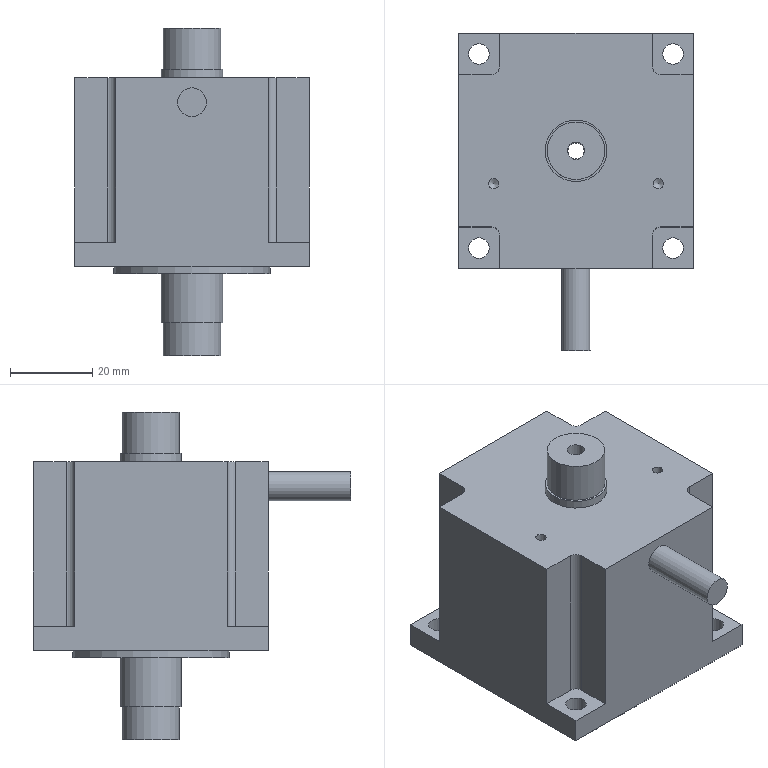Part | NX | 1 solid | 45 faces | box 57 x 77 x 79.6 mm | volume 139845 mm3 | plane 24 | cylinder 18 | cone 3 | commonest cylinder face diameters 4 x5 5 x4 2.5 x2 14 x2 15 x2 4.2 x1
STEP:
#1=CARTESIAN_POINT('',(18.5,-28.5,6.));
#2=VERTEX_POINT('',#1);
#3=CARTESIAN_POINT('',(28.5,-28.5,6.));
#4=VERTEX_POINT('',#3);
#5=CARTESIAN_POINT('',(28.5,-28.5,6.));
#6=DIRECTION('',(1.,0.,0.));
#7=VECTOR('',#6,1000.);
#8=LINE('',#5,#7);
#9=EDGE_CURVE('',#2,#4,#8,.T.);
#10=ORIENTED_EDGE('',*,*,#9,.F.);
#11=CARTESIAN_POINT('',(18.5,-28.5,46.));
#12=VERTEX_POINT('',#11);
#13=CARTESIAN_POINT('',(18.5,-28.5,6.));
#14=DIRECTION('',(0.,0.,1.));
#15=VECTOR('',#14,1000.);
#16=LINE('',#13,#15);
#17=EDGE_CURVE('',#2,#12,#16,.T.);
#18=ORIENTED_EDGE('',*,*,#17,.T.);
#19=CARTESIAN_POINT('',(-18.5,-28.5,46.));
#20=VERTEX_POINT('',#19);
#21=CARTESIAN_POINT('',(-28.5,-28.5,46.));
#22=DIRECTION('',(1.,0.,0.));
#23=VECTOR('',#22,1000.);
#24=LINE('',#21,#23);
#25=EDGE_CURVE('',#20,#12,#24,.T.);
#26=ORIENTED_EDGE('',*,*,#25,.F.);
#27=CARTESIAN_POINT('',(-18.5,-28.5,6.));
#28=VERTEX_POINT('',#27);
#29=CARTESIAN_POINT('',(-18.5,-28.5,6.));
#30=DIRECTION('',(0.,0.,1.));
#31=VECTOR('',#30,1000.);
#32=LINE('',#29,#31);
#33=EDGE_CURVE('',#28,#20,#32,.T.);
#34=ORIENTED_EDGE('',*,*,#33,.F.);
#35=CARTESIAN_POINT('',(-28.5,-28.5,6.));
#36=VERTEX_POINT('',#35);
#37=CARTESIAN_POINT('',(-28.5,-28.5,6.));
#38=DIRECTION('',(1.,0.,0.));
#39=VECTOR('',#38,1000.);
#40=LINE('',#37,#39);
#41=EDGE_CURVE('',#36,#28,#40,.T.);
#42=ORIENTED_EDGE('',*,*,#41,.F.);
#43=CARTESIAN_POINT('',(-28.5,-28.5,0.));
#44=VERTEX_POINT('',#43);
#45=CARTESIAN_POINT('',(-28.5,-28.5,46.));
#46=DIRECTION('',(0.,0.,-1.));
#47=VECTOR('',#46,1000.);
#48=LINE('',#45,#47);
#49=EDGE_CURVE('',#36,#44,#48,.T.);
#50=ORIENTED_EDGE('',*,*,#49,.T.);
#51=CARTESIAN_POINT('',(28.5,-28.5,0.));
#52=VERTEX_POINT('',#51);
#53=CARTESIAN_POINT('',(-28.5,-28.5,0.));
#54=DIRECTION('',(1.,0.,0.));
#55=VECTOR('',#54,1000.);
#56=LINE('',#53,#55);
#57=EDGE_CURVE('',#44,#52,#56,.T.);
#58=ORIENTED_EDGE('',*,*,#57,.T.);
#59=CARTESIAN_POINT('',(28.5,-28.5,46.));
#60=DIRECTION('',(0.,0.,-1.));
#61=VECTOR('',#60,1000.);
#62=LINE('',#59,#61);
#63=EDGE_CURVE('',#4,#52,#62,.T.);
#64=ORIENTED_EDGE('',*,*,#63,.F.);
#65=EDGE_LOOP('',(#10,#18,#26,#34,#42,#50,#58,#64));
#66=FACE_BOUND('',#65,.T.);
#67=CARTESIAN_POINT('',(0.,-28.5,43.5));
#68=VERTEX_POINT('',#67);
#69=CARTESIAN_POINT('',(0.,-28.5,40.));
#70=DIRECTION('',(0.,1.,0.));
#71=DIRECTION('',(0.,0.,1.));
#72=AXIS2_PLACEMENT_3D('',#69,#70,#71);
#73=CIRCLE('',#72,3.5);
#74=EDGE_CURVE('',#68,#68,#73,.F.);
#75=ORIENTED_EDGE('',*,*,#74,.F.);
#76=EDGE_LOOP('',(#75));
#77=FACE_BOUND('',#76,.T.);
#78=CARTESIAN_POINT('',(-28.5,-28.5,46.));
#79=DIRECTION('',(0.,1.,0.));
#80=DIRECTION('',(0.,0.,1.));
#81=AXIS2_PLACEMENT_3D('',#78,#79,#80);
#82=PLANE('',#81);
#83=ADVANCED_FACE('',(#66,#77),#82,.F.);
#84=CARTESIAN_POINT('',(-7.5,0.,-1.6));
#85=VERTEX_POINT('',#84);
#86=CARTESIAN_POINT('',(0.,0.,-1.6));
#87=DIRECTION('',(0.,0.,-1.));
#88=DIRECTION('',(-1.,0.,0.));
#89=AXIS2_PLACEMENT_3D('',#86,#87,#88);
#90=CIRCLE('',#89,7.5);
#91=EDGE_CURVE('',#85,#85,#90,.T.);
#92=ORIENTED_EDGE('',*,*,#91,.T.);
#93=EDGE_LOOP('',(#92));
#94=FACE_BOUND('',#93,.T.);
#95=CARTESIAN_POINT('',(-7.5,0.,-13.6));
#96=VERTEX_POINT('',#95);
#97=CARTESIAN_POINT('',(0.,0.,-13.6));
#98=DIRECTION('',(0.,0.,-1.));
#99=DIRECTION('',(-1.,0.,0.));
#100=AXIS2_PLACEMENT_3D('',#97,#98,#99);
#101=CIRCLE('',#100,7.5);
#102=EDGE_CURVE('',#96,#96,#101,.T.);
#103=ORIENTED_EDGE('',*,*,#102,.F.);
#104=EDGE_LOOP('',(#103));
#105=FACE_BOUND('',#104,.T.);
#106=CARTESIAN_POINT('',(0.,0.,-21.6));
#107=DIRECTION('',(0.,0.,1.));
#108=DIRECTION('',(1.,0.,0.));
#109=AXIS2_PLACEMENT_3D('',#106,#107,#108);
#110=CYLINDRICAL_SURFACE('',#109,7.5);
#111=ADVANCED_FACE('',(#94,#105),#110,.T.);
#112=CARTESIAN_POINT('',(-2.,0.,-21.6));
#113=VERTEX_POINT('',#112);
#114=CARTESIAN_POINT('',(0.,0.,-21.6));
#115=DIRECTION('',(0.,0.,-1.));
#116=DIRECTION('',(-1.,0.,0.));
#117=AXIS2_PLACEMENT_3D('',#114,#115,#116);
#118=CIRCLE('',#117,2.);
#119=EDGE_CURVE('',#113,#113,#118,.T.);
#120=ORIENTED_EDGE('',*,*,#119,.F.);
#121=EDGE_LOOP('',(#120));
#122=FACE_BOUND('',#121,.T.);
#123=CARTESIAN_POINT('',(-7.,0.,-21.6));
#124=VERTEX_POINT('',#123);
#125=CARTESIAN_POINT('',(0.,0.,-21.6));
#126=DIRECTION('',(0.,0.,-1.));
#127=DIRECTION('',(-1.,0.,0.));
#128=AXIS2_PLACEMENT_3D('',#125,#126,#127);
#129=CIRCLE('',#128,7.);
#130=EDGE_CURVE('',#124,#124,#129,.T.);
#131=ORIENTED_EDGE('',*,*,#130,.T.);
#132=EDGE_LOOP('',(#131));
#133=FACE_BOUND('',#132,.T.);
#134=CARTESIAN_POINT('',(0.,0.,-21.6));
#135=DIRECTION('',(0.,0.,-1.));
#136=DIRECTION('',(-1.,0.,0.));
#137=AXIS2_PLACEMENT_3D('',#134,#135,#136);
#138=PLANE('',#137);
#139=ADVANCED_FACE('',(#122,#133),#138,.T.);
#140=CARTESIAN_POINT('',(7.5,0.,48.));
#141=VERTEX_POINT('',#140);
#142=CARTESIAN_POINT('',(0.,0.,48.));
#143=DIRECTION('',(0.,0.,1.));
#144=DIRECTION('',(1.,0.,0.));
#145=AXIS2_PLACEMENT_3D('',#142,#143,#144);
#146=CIRCLE('',#145,7.5);
#147=EDGE_CURVE('',#141,#141,#146,.T.);
#148=ORIENTED_EDGE('',*,*,#147,.T.);
#149=EDGE_LOOP('',(#148));
#150=FACE_BOUND('',#149,.T.);
#151=CARTESIAN_POINT('',(7.,0.,48.));
#152=VERTEX_POINT('',#151);
#153=CARTESIAN_POINT('',(0.,0.,48.));
#154=DIRECTION('',(0.,0.,1.));
#155=DIRECTION('',(1.,0.,0.));
#156=AXIS2_PLACEMENT_3D('',#153,#154,#155);
#157=CIRCLE('',#156,7.);
#158=EDGE_CURVE('',#152,#152,#157,.T.);
#159=ORIENTED_EDGE('',*,*,#158,.F.);
#160=EDGE_LOOP('',(#159));
#161=FACE_BOUND('',#160,.T.);
#162=CARTESIAN_POINT('',(0.,0.,48.));
#163=DIRECTION('',(0.,0.,1.));
#164=DIRECTION('',(1.,0.,0.));
#165=AXIS2_PLACEMENT_3D('',#162,#163,#164);
#166=PLANE('',#165);
#167=ADVANCED_FACE('',(#150,#161),#166,.T.);
#168=CARTESIAN_POINT('',(-18.75,-8.,46.));
#169=VERTEX_POINT('',#168);
#170=CARTESIAN_POINT('',(-20.,-8.,46.));
#171=DIRECTION('',(0.,0.,1.));
#172=DIRECTION('',(1.,0.,0.));
#173=AXIS2_PLACEMENT_3D('',#170,#171,#172);
#174=CIRCLE('',#173,1.25);
#175=EDGE_CURVE('',#169,#169,#174,.T.);
#176=ORIENTED_EDGE('',*,*,#175,.F.);
#177=EDGE_LOOP('',(#176));
#178=FACE_BOUND('',#177,.T.);
#179=CARTESIAN_POINT('',(21.25,-8.,46.));
#180=VERTEX_POINT('',#179);
#181=CARTESIAN_POINT('',(20.,-8.,46.));
#182=DIRECTION('',(0.,0.,1.));
#183=DIRECTION('',(1.,0.,0.));
#184=AXIS2_PLACEMENT_3D('',#181,#182,#183);
#185=CIRCLE('',#184,1.25);
#186=EDGE_CURVE('',#180,#180,#185,.T.);
#187=ORIENTED_EDGE('',*,*,#186,.F.);
#188=EDGE_LOOP('',(#187));
#189=FACE_BOUND('',#188,.T.);
#190=ORIENTED_EDGE('',*,*,#25,.T.);
#191=CARTESIAN_POINT('',(18.5,-20.5,46.));
#192=VERTEX_POINT('',#191);
#193=CARTESIAN_POINT('',(18.5,-28.5,46.));
#194=DIRECTION('',(0.,-1.,0.));
#195=VECTOR('',#194,1000.);
#196=LINE('',#193,#195);
#197=EDGE_CURVE('',#192,#12,#196,.T.);
#198=ORIENTED_EDGE('',*,*,#197,.F.);
#199=CARTESIAN_POINT('',(20.5,-18.5,46.));
#200=VERTEX_POINT('',#199);
#201=CARTESIAN_POINT('',(20.5,-20.5,46.));
#202=DIRECTION('',(0.,0.,-1.));
#203=DIRECTION('',(-1.,0.,0.));
#204=AXIS2_PLACEMENT_3D('',#201,#202,#203);
#205=CIRCLE('',#204,2.);
#206=EDGE_CURVE('',#192,#200,#205,.T.);
#207=ORIENTED_EDGE('',*,*,#206,.T.);
#208=CARTESIAN_POINT('',(28.5,-18.5,46.));
#209=VERTEX_POINT('',#208);
#210=CARTESIAN_POINT('',(28.5,-18.5,46.));
#211=DIRECTION('',(-1.,0.,0.));
#212=VECTOR('',#211,1000.);
#213=LINE('',#210,#212);
#214=EDGE_CURVE('',#209,#200,#213,.T.);
#215=ORIENTED_EDGE('',*,*,#214,.F.);
#216=CARTESIAN_POINT('',(28.5,18.5,46.));
#217=VERTEX_POINT('',#216);
#218=CARTESIAN_POINT('',(28.5,-28.5,46.));
#219=DIRECTION('',(0.,1.,0.));
#220=VECTOR('',#219,1000.);
#221=LINE('',#218,#220);
#222=EDGE_CURVE('',#209,#217,#221,.T.);
#223=ORIENTED_EDGE('',*,*,#222,.T.);
#224=CARTESIAN_POINT('',(20.5,18.5,46.));
#225=VERTEX_POINT('',#224);
#226=CARTESIAN_POINT('',(28.5,18.5,46.));
#227=DIRECTION('',(1.,0.,0.));
#228=VECTOR('',#227,1000.);
#229=LINE('',#226,#228);
#230=EDGE_CURVE('',#225,#217,#229,.T.);
#231=ORIENTED_EDGE('',*,*,#230,.F.);
#232=CARTESIAN_POINT('',(18.5,20.5,46.));
#233=VERTEX_POINT('',#232);
#234=CARTESIAN_POINT('',(20.5,20.5,46.));
#235=DIRECTION('',(0.,0.,-1.));
#236=DIRECTION('',(-1.,0.,0.));
#237=AXIS2_PLACEMENT_3D('',#234,#235,#236);
#238=CIRCLE('',#237,2.);
#239=EDGE_CURVE('',#225,#233,#238,.T.);
#240=ORIENTED_EDGE('',*,*,#239,.T.);
#241=CARTESIAN_POINT('',(18.5,28.5,46.));
#242=VERTEX_POINT('',#241);
#243=CARTESIAN_POINT('',(18.5,28.5,46.));
#244=DIRECTION('',(0.,-1.,0.));
#245=VECTOR('',#244,1000.);
#246=LINE('',#243,#245);
#247=EDGE_CURVE('',#242,#233,#246,.T.);
#248=ORIENTED_EDGE('',*,*,#247,.F.);
#249=CARTESIAN_POINT('',(-18.5,28.5,46.));
#250=VERTEX_POINT('',#249);
#251=CARTESIAN_POINT('',(-28.5,28.5,46.));
#252=DIRECTION('',(-1.,0.,0.));
#253=VECTOR('',#252,1000.);
#254=LINE('',#251,#253);
#255=EDGE_CURVE('',#242,#250,#254,.T.);
#256=ORIENTED_EDGE('',*,*,#255,.T.);
#257=CARTESIAN_POINT('',(-18.5,20.5,46.));
#258=VERTEX_POINT('',#257);
#259=CARTESIAN_POINT('',(-18.5,28.5,46.));
#260=DIRECTION('',(0.,1.,0.));
#261=VECTOR('',#260,1000.);
#262=LINE('',#259,#261);
#263=EDGE_CURVE('',#258,#250,#262,.T.);
#264=ORIENTED_EDGE('',*,*,#263,.F.);
#265=CARTESIAN_POINT('',(-20.5,18.5,46.));
#266=VERTEX_POINT('',#265);
#267=CARTESIAN_POINT('',(-20.5,20.5,46.));
#268=DIRECTION('',(0.,0.,-1.));
#269=DIRECTION('',(-1.,0.,0.));
#270=AXIS2_PLACEMENT_3D('',#267,#268,#269);
#271=CIRCLE('',#270,2.);
#272=EDGE_CURVE('',#258,#266,#271,.T.);
#273=ORIENTED_EDGE('',*,*,#272,.T.);
#274=CARTESIAN_POINT('',(-28.5,18.5,46.));
#275=VERTEX_POINT('',#274);
#276=CARTESIAN_POINT('',(-28.5,18.5,46.));
#277=DIRECTION('',(1.,0.,0.));
#278=VECTOR('',#277,1000.);
#279=LINE('',#276,#278);
#280=EDGE_CURVE('',#275,#266,#279,.T.);
#281=ORIENTED_EDGE('',*,*,#280,.F.);
#282=CARTESIAN_POINT('',(-28.5,-18.5,46.));
#283=VERTEX_POINT('',#282);
#284=CARTESIAN_POINT('',(-28.5,-28.5,46.));
#285=DIRECTION('',(0.,-1.,0.));
#286=VECTOR('',#285,1000.);
#287=LINE('',#284,#286);
#288=EDGE_CURVE('',#275,#283,#287,.T.);
#289=ORIENTED_EDGE('',*,*,#288,.T.);
#290=CARTESIAN_POINT('',(-20.5,-18.5,46.));
#291=VERTEX_POINT('',#290);
#292=CARTESIAN_POINT('',(-28.5,-18.5,46.));
#293=DIRECTION('',(-1.,0.,0.));
#294=VECTOR('',#293,1000.);
#295=LINE('',#292,#294);
#296=EDGE_CURVE('',#291,#283,#295,.T.);
#297=ORIENTED_EDGE('',*,*,#296,.F.);
#298=CARTESIAN_POINT('',(-18.5,-20.5,46.));
#299=VERTEX_POINT('',#298);
#300=CARTESIAN_POINT('',(-20.5,-20.5,46.));
#301=DIRECTION('',(0.,0.,-1.));
#302=DIRECTION('',(-1.,0.,0.));
#303=AXIS2_PLACEMENT_3D('',#300,#301,#302);
#304=CIRCLE('',#303,2.);
#305=EDGE_CURVE('',#291,#299,#304,.T.);
#306=ORIENTED_EDGE('',*,*,#305,.T.);
#307=CARTESIAN_POINT('',(-18.5,-28.5,46.));
#308=DIRECTION('',(0.,1.,0.));
#309=VECTOR('',#308,1000.);
#310=LINE('',#307,#309);
#311=EDGE_CURVE('',#20,#299,#310,.T.);
#312=ORIENTED_EDGE('',*,*,#311,.F.);
#313=EDGE_LOOP('',(#190,#198,#207,#215,#223,#231,#240,#248,#256,#264,#273,#281,#289,#297,#306,#312));
#314=FACE_BOUND('',#313,.T.);
#315=CARTESIAN_POINT('',(-7.5,0.,46.));
#316=VERTEX_POINT('',#315);
#317=CARTESIAN_POINT('',(0.,0.,46.));
#318=DIRECTION('',(0.,0.,-1.));
#319=DIRECTION('',(-1.,0.,0.));
#320=AXIS2_PLACEMENT_3D('',#317,#318,#319);
#321=CIRCLE('',#320,7.5);
#322=EDGE_CURVE('',#316,#316,#321,.F.);
#323=ORIENTED_EDGE('',*,*,#322,.F.);
#324=EDGE_LOOP('',(#323));
#325=FACE_BOUND('',#324,.T.);
#326=CARTESIAN_POINT('',(0.,0.,46.));
#327=DIRECTION('',(0.,0.,-1.));
#328=DIRECTION('',(-1.,0.,0.));
#329=AXIS2_PLACEMENT_3D('',#326,#327,#328);
#330=PLANE('',#329);
#331=ADVANCED_FACE('',(#178,#189,#314,#325),#330,.F.);
#332=CARTESIAN_POINT('',(-19.,0.,-1.6));
#333=VERTEX_POINT('',#332);
#334=CARTESIAN_POINT('',(0.,0.,-1.6));
#335=DIRECTION('',(0.,0.,-1.));
#336=DIRECTION('',(-1.,0.,0.));
#337=AXIS2_PLACEMENT_3D('',#334,#335,#336);
#338=CIRCLE('',#337,19.);
#339=EDGE_CURVE('',#333,#333,#338,.T.);
#340=ORIENTED_EDGE('',*,*,#339,.T.);
#341=EDGE_LOOP('',(#340));
#342=FACE_BOUND('',#341,.T.);
#343=ORIENTED_EDGE('',*,*,#91,.F.);
#344=EDGE_LOOP('',(#343));
#345=FACE_BOUND('',#344,.T.);
#346=CARTESIAN_POINT('',(0.,0.,-1.6));
#347=DIRECTION('',(0.,0.,-1.));
#348=DIRECTION('',(-1.,0.,0.));
#349=AXIS2_PLACEMENT_3D('',#346,#347,#348);
#350=PLANE('',#349);
#351=ADVANCED_FACE('',(#342,#345),#350,.T.);
#352=CARTESIAN_POINT('',(-26.07,23.57,0.));
#353=VERTEX_POINT('',#352);
#354=CARTESIAN_POINT('',(-23.57,23.57,0.));
#355=DIRECTION('',(0.,0.,-1.));
#356=DIRECTION('',(-1.,0.,0.));
#357=AXIS2_PLACEMENT_3D('',#354,#355,#356);
#358=CIRCLE('',#357,2.5);
#359=EDGE_CURVE('',#353,#353,#358,.T.);
#360=ORIENTED_EDGE('',*,*,#359,.F.);
#361=EDGE_LOOP('',(#360));
#362=FACE_BOUND('',#361,.T.);
#363=CARTESIAN_POINT('',(21.07,23.57,0.));
#364=VERTEX_POINT('',#363);
#365=CARTESIAN_POINT('',(23.57,23.57,0.));
#366=DIRECTION('',(0.,0.,-1.));
#367=DIRECTION('',(-1.,0.,0.));
#368=AXIS2_PLACEMENT_3D('',#365,#366,#367);
#369=CIRCLE('',#368,2.5);
#370=EDGE_CURVE('',#364,#364,#369,.T.);
#371=ORIENTED_EDGE('',*,*,#370,.F.);
#372=EDGE_LOOP('',(#371));
#373=FACE_BOUND('',#372,.T.);
#374=CARTESIAN_POINT('',(21.07,-23.57,0.));
#375=VERTEX_POINT('',#374);
#376=CARTESIAN_POINT('',(23.57,-23.57,0.));
#377=DIRECTION('',(0.,0.,-1.));
#378=DIRECTION('',(-1.,0.,0.));
#379=AXIS2_PLACEMENT_3D('',#376,#377,#378);
#380=CIRCLE('',#379,2.5);
#381=EDGE_CURVE('',#375,#375,#380,.T.);
#382=ORIENTED_EDGE('',*,*,#381,.F.);
#383=EDGE_LOOP('',(#382));
#384=FACE_BOUND('',#383,.T.);
#385=CARTESIAN_POINT('',(-26.07,-23.57,0.));
#386=VERTEX_POINT('',#385);
#387=CARTESIAN_POINT('',(-23.57,-23.57,0.));
#388=DIRECTION('',(0.,0.,-1.));
#389=DIRECTION('',(-1.,0.,0.));
#390=AXIS2_PLACEMENT_3D('',#387,#388,#389);
#391=CIRCLE('',#390,2.5);
#392=EDGE_CURVE('',#386,#386,#391,.T.);
#393=ORIENTED_EDGE('',*,*,#392,.F.);
#394=EDGE_LOOP('',(#393));
#395=FACE_BOUND('',#394,.T.);
#396=CARTESIAN_POINT('',(28.5,28.5,0.));
#397=VERTEX_POINT('',#396);
#398=CARTESIAN_POINT('',(28.5,-28.5,0.));
#399=DIRECTION('',(0.,1.,0.));
#400=VECTOR('',#399,1000.);
#401=LINE('',#398,#400);
#402=EDGE_CURVE('',#52,#397,#401,.T.);
#403=ORIENTED_EDGE('',*,*,#402,.F.);
#404=ORIENTED_EDGE('',*,*,#57,.F.);
#405=CARTESIAN_POINT('',(-28.5,28.5,0.));
#406=VERTEX_POINT('',#405);
#407=CARTESIAN_POINT('',(-28.5,-28.5,0.));
#408=DIRECTION('',(0.,-1.,0.));
#409=VECTOR('',#408,1000.);
#410=LINE('',#407,#409);
#411=EDGE_CURVE('',#406,#44,#410,.T.);
#412=ORIENTED_EDGE('',*,*,#411,.F.);
#413=CARTESIAN_POINT('',(-28.5,28.5,0.));
#414=DIRECTION('',(-1.,0.,0.));
#415=VECTOR('',#414,1000.);
#416=LINE('',#413,#415);
#417=EDGE_CURVE('',#397,#406,#416,.T.);
#418=ORIENTED_EDGE('',*,*,#417,.F.);
#419=EDGE_LOOP('',(#403,#404,#412,#418));
#420=FACE_BOUND('',#419,.T.);
#421=CARTESIAN_POINT('',(-19.,0.,0.));
#422=VERTEX_POINT('',#421);
#423=CARTESIAN_POINT('',(0.,0.,0.));
#424=DIRECTION('',(0.,0.,-1.));
#425=DIRECTION('',(-1.,0.,0.));
#426=AXIS2_PLACEMENT_3D('',#423,#424,#425);
#427=CIRCLE('',#426,19.);
#428=EDGE_CURVE('',#422,#422,#427,.T.);
#429=ORIENTED_EDGE('',*,*,#428,.F.);
#430=EDGE_LOOP('',(#429));
#431=FACE_BOUND('',#430,.T.);
#432=CARTESIAN_POINT('',(0.,0.,0.));
#433=DIRECTION('',(0.,0.,-1.));
#434=DIRECTION('',(-1.,0.,0.));
#435=AXIS2_PLACEMENT_3D('',#432,#433,#434);
#436=PLANE('',#435);
#437=ADVANCED_FACE('',(#362,#373,#384,#395,#420,#431),#436,.T.);
#438=ORIENTED_EDGE('',*,*,#222,.F.);
#439=CARTESIAN_POINT('',(28.5,-18.5,6.));
#440=VERTEX_POINT('',#439);
#441=CARTESIAN_POINT('',(28.5,-18.5,6.));
#442=DIRECTION('',(0.,0.,1.));
#443=VECTOR('',#442,1000.);
#444=LINE('',#441,#443);
#445=EDGE_CURVE('',#440,#209,#444,.T.);
#446=ORIENTED_EDGE('',*,*,#445,.F.);
#447=CARTESIAN_POINT('',(28.5,-28.5,6.));
#448=DIRECTION('',(0.,1.,0.));
#449=VECTOR('',#448,1000.);
#450=LINE('',#447,#449);
#451=EDGE_CURVE('',#4,#440,#450,.T.);
#452=ORIENTED_EDGE('',*,*,#451,.F.);
#453=ORIENTED_EDGE('',*,*,#63,.T.);
#454=ORIENTED_EDGE('',*,*,#402,.T.);
#455=CARTESIAN_POINT('',(28.5,28.5,6.));
#456=VERTEX_POINT('',#455);
#457=CARTESIAN_POINT('',(28.5,28.5,46.));
#458=DIRECTION('',(0.,0.,-1.));
#459=VECTOR('',#458,1000.);
#460=LINE('',#457,#459);
#461=EDGE_CURVE('',#456,#397,#460,.T.);
#462=ORIENTED_EDGE('',*,*,#461,.F.);
#463=CARTESIAN_POINT('',(28.5,18.5,6.));
#464=VERTEX_POINT('',#463);
#465=CARTESIAN_POINT('',(28.5,28.5,6.));
#466=DIRECTION('',(0.,1.,0.));
#467=VECTOR('',#466,1000.);
#468=LINE('',#465,#467);
#469=EDGE_CURVE('',#464,#456,#468,.T.);
#470=ORIENTED_EDGE('',*,*,#469,.F.);
#471=CARTESIAN_POINT('',(28.5,18.5,6.));
#472=DIRECTION('',(0.,0.,1.));
#473=VECTOR('',#472,1000.);
#474=LINE('',#471,#473);
#475=EDGE_CURVE('',#464,#217,#474,.T.);
#476=ORIENTED_EDGE('',*,*,#475,.T.);
#477=EDGE_LOOP('',(#438,#446,#452,#453,#454,#462,#470,#476));
#478=FACE_BOUND('',#477,.T.);
#479=CARTESIAN_POINT('',(28.5,-28.5,46.));
#480=DIRECTION('',(-1.,0.,0.));
#481=DIRECTION('',(0.,0.,1.));
#482=AXIS2_PLACEMENT_3D('',#479,#480,#481);
#483=PLANE('',#482);
#484=ADVANCED_FACE('',(#478),#483,.F.);
#485=CARTESIAN_POINT('',(-18.5,28.5,6.));
#486=VERTEX_POINT('',#485);
#487=CARTESIAN_POINT('',(-28.5,28.5,6.));
#488=VERTEX_POINT('',#487);
#489=CARTESIAN_POINT('',(-28.5,28.5,6.));
#490=DIRECTION('',(-1.,0.,0.));
#491=VECTOR('',#490,1000.);
#492=LINE('',#489,#491);
#493=EDGE_CURVE('',#486,#488,#492,.T.);
#494=ORIENTED_EDGE('',*,*,#493,.F.);
#495=CARTESIAN_POINT('',(-18.5,28.5,6.));
#496=DIRECTION('',(0.,0.,1.));
#497=VECTOR('',#496,1000.);
#498=LINE('',#495,#497);
#499=EDGE_CURVE('',#486,#250,#498,.T.);
#500=ORIENTED_EDGE('',*,*,#499,.T.);
#501=ORIENTED_EDGE('',*,*,#255,.F.);
#502=CARTESIAN_POINT('',(18.5,28.5,6.));
#503=VERTEX_POINT('',#502);
#504=CARTESIAN_POINT('',(18.5,28.5,6.));
#505=DIRECTION('',(0.,0.,1.));
#506=VECTOR('',#505,1000.);
#507=LINE('',#504,#506);
#508=EDGE_CURVE('',#503,#242,#507,.T.);
#509=ORIENTED_EDGE('',*,*,#508,.F.);
#510=CARTESIAN_POINT('',(28.5,28.5,6.));
#511=DIRECTION('',(-1.,0.,0.));
#512=VECTOR('',#511,1000.);
#513=LINE('',#510,#512);
#514=EDGE_CURVE('',#456,#503,#513,.T.);
#515=ORIENTED_EDGE('',*,*,#514,.F.);
#516=ORIENTED_EDGE('',*,*,#461,.T.);
#517=ORIENTED_EDGE('',*,*,#417,.T.);
#518=CARTESIAN_POINT('',(-28.5,28.5,46.));
#519=DIRECTION('',(0.,0.,-1.));
#520=VECTOR('',#519,1000.);
#521=LINE('',#518,#520);
#522=EDGE_CURVE('',#488,#406,#521,.T.);
#523=ORIENTED_EDGE('',*,*,#522,.F.);
#524=EDGE_LOOP('',(#494,#500,#501,#509,#515,#516,#517,#523));
#525=FACE_BOUND('',#524,.T.);
#526=CARTESIAN_POINT('',(-28.5,28.5,46.));
#527=DIRECTION('',(0.,-1.,0.));
#528=DIRECTION('',(0.,0.,-1.));
#529=AXIS2_PLACEMENT_3D('',#526,#527,#528);
#530=PLANE('',#529);
#531=ADVANCED_FACE('',(#525),#530,.F.);
#532=CARTESIAN_POINT('',(-28.5,-18.5,6.));
#533=VERTEX_POINT('',#532);
#534=CARTESIAN_POINT('',(-28.5,-28.5,6.));
#535=DIRECTION('',(0.,-1.,0.));
#536=VECTOR('',#535,1000.);
#537=LINE('',#534,#536);
#538=EDGE_CURVE('',#533,#36,#537,.T.);
#539=ORIENTED_EDGE('',*,*,#538,.F.);
#540=CARTESIAN_POINT('',(-28.5,-18.5,6.));
#541=DIRECTION('',(0.,0.,1.));
#542=VECTOR('',#541,1000.);
#543=LINE('',#540,#542);
#544=EDGE_CURVE('',#533,#283,#543,.T.);
#545=ORIENTED_EDGE('',*,*,#544,.T.);
#546=ORIENTED_EDGE('',*,*,#288,.F.);
#547=CARTESIAN_POINT('',(-28.5,18.5,6.));
#548=VERTEX_POINT('',#547);
#549=CARTESIAN_POINT('',(-28.5,18.5,6.));
#550=DIRECTION('',(0.,0.,1.));
#551=VECTOR('',#550,1000.);
#552=LINE('',#549,#551);
#553=EDGE_CURVE('',#548,#275,#552,.T.);
#554=ORIENTED_EDGE('',*,*,#553,.F.);
#555=CARTESIAN_POINT('',(-28.5,28.5,6.));
#556=DIRECTION('',(0.,-1.,0.));
#557=VECTOR('',#556,1000.);
#558=LINE('',#555,#557);
#559=EDGE_CURVE('',#488,#548,#558,.T.);
#560=ORIENTED_EDGE('',*,*,#559,.F.);
#561=ORIENTED_EDGE('',*,*,#522,.T.);
#562=ORIENTED_EDGE('',*,*,#411,.T.);
#563=ORIENTED_EDGE('',*,*,#49,.F.);
#564=EDGE_LOOP('',(#539,#545,#546,#554,#560,#561,#562,#563));
#565=FACE_BOUND('',#564,.T.);
#566=CARTESIAN_POINT('',(-28.5,-28.5,46.));
#567=DIRECTION('',(1.,0.,0.));
#568=DIRECTION('',(0.,0.,-1.));
#569=AXIS2_PLACEMENT_3D('',#566,#567,#568);
#570=PLANE('',#569);
#571=ADVANCED_FACE('',(#565),#570,.F.);
#572=ORIENTED_EDGE('',*,*,#339,.F.);
#573=EDGE_LOOP('',(#572));
#574=FACE_BOUND('',#573,.T.);
#575=ORIENTED_EDGE('',*,*,#428,.T.);
#576=EDGE_LOOP('',(#575));
#577=FACE_BOUND('',#576,.T.);
#578=CARTESIAN_POINT('',(0.,0.,-1.6));
#579=DIRECTION('',(0.,0.,1.));
#580=DIRECTION('',(1.,0.,0.));
#581=AXIS2_PLACEMENT_3D('',#578,#579,#580);
#582=CYLINDRICAL_SURFACE('',#581,19.);
#583=ADVANCED_FACE('',(#574,#577),#582,.T.);
#584=ORIENTED_EDGE('',*,*,#147,.F.);
#585=EDGE_LOOP('',(#584));
#586=FACE_BOUND('',#585,.T.);
#587=ORIENTED_EDGE('',*,*,#322,.T.);
#588=EDGE_LOOP('',(#587));
#589=FACE_BOUND('',#588,.T.);
#590=CARTESIAN_POINT('',(0.,0.,48.));
#591=DIRECTION('',(0.,0.,-1.));
#592=DIRECTION('',(-1.,0.,0.));
#593=AXIS2_PLACEMENT_3D('',#590,#591,#592);
#594=CYLINDRICAL_SURFACE('',#593,7.5);
#595=ADVANCED_FACE('',(#586,#589),#594,.T.);
#596=CARTESIAN_POINT('',(7.,0.,58.));
#597=VERTEX_POINT('',#596);
#598=CARTESIAN_POINT('',(0.,0.,58.));
#599=DIRECTION('',(0.,0.,1.));
#600=DIRECTION('',(1.,0.,0.));
#601=AXIS2_PLACEMENT_3D('',#598,#599,#600);
#602=CIRCLE('',#601,7.);
#603=EDGE_CURVE('',#597,#597,#602,.T.);
#604=ORIENTED_EDGE('',*,*,#603,.F.);
#605=EDGE_LOOP('',(#604));
#606=FACE_BOUND('',#605,.T.);
#607=ORIENTED_EDGE('',*,*,#158,.T.);
#608=EDGE_LOOP('',(#607));
#609=FACE_BOUND('',#608,.T.);
#610=CARTESIAN_POINT('',(0.,0.,58.));
#611=DIRECTION('',(0.,0.,-1.));
#612=DIRECTION('',(-1.,0.,0.));
#613=AXIS2_PLACEMENT_3D('',#610,#611,#612);
#614=CYLINDRICAL_SURFACE('',#613,7.);
#615=ADVANCED_FACE('',(#606,#609),#614,.T.);
#616=CARTESIAN_POINT('',(2.1,0.,58.));
#617=VERTEX_POINT('',#616);
#618=CARTESIAN_POINT('',(0.,0.,58.));
#619=DIRECTION('',(0.,0.,1.));
#620=DIRECTION('',(1.,0.,0.));
#621=AXIS2_PLACEMENT_3D('',#618,#619,#620);
#622=CIRCLE('',#621,2.1);
#623=EDGE_CURVE('',#617,#617,#622,.T.);
#624=ORIENTED_EDGE('',*,*,#623,.F.);
#625=EDGE_LOOP('',(#624));
#626=FACE_BOUND('',#625,.T.);
#627=ORIENTED_EDGE('',*,*,#603,.T.);
#628=EDGE_LOOP('',(#627));
#629=FACE_BOUND('',#628,.T.);
#630=CARTESIAN_POINT('',(0.,0.,58.));
#631=DIRECTION('',(0.,0.,1.));
#632=DIRECTION('',(1.,0.,0.));
#633=AXIS2_PLACEMENT_3D('',#630,#631,#632);
#634=PLANE('',#633);
#635=ADVANCED_FACE('',(#626,#629),#634,.T.);
#636=CARTESIAN_POINT('',(2.,0.,43.94));
#637=VERTEX_POINT('',#636);
#638=CARTESIAN_POINT('',(0.,0.,43.94));
#639=DIRECTION('',(0.,0.,1.));
#640=DIRECTION('',(1.,0.,0.));
#641=AXIS2_PLACEMENT_3D('',#638,#639,#640);
#642=CIRCLE('',#641,2.);
#643=EDGE_CURVE('',#637,#637,#642,.F.);
#644=ORIENTED_EDGE('',*,*,#643,.T.);
#645=EDGE_LOOP('',(#644));
#646=FACE_BOUND('',#645,.T.);
#647=CARTESIAN_POINT('',(2.1,0.,44.));
#648=VERTEX_POINT('',#647);
#649=CARTESIAN_POINT('',(0.,0.,44.));
#650=DIRECTION('',(0.,0.,1.));
#651=DIRECTION('',(1.,0.,0.));
#652=AXIS2_PLACEMENT_3D('',#649,#650,#651);
#653=CIRCLE('',#652,2.1);
#654=EDGE_CURVE('',#648,#648,#653,.T.);
#655=ORIENTED_EDGE('',*,*,#654,.T.);
#656=EDGE_LOOP('',(#655));
#657=FACE_BOUND('',#656,.T.);
#658=CARTESIAN_POINT('',(0.,0.,44.));
#659=DIRECTION('',(0.,0.,1.));
#660=DIRECTION('',(1.,0.,0.));
#661=AXIS2_PLACEMENT_3D('',#658,#659,#660);
#662=CONICAL_SURFACE('',#661,2.1,1.03);
#663=ADVANCED_FACE('',(#646,#657),#662,.F.);
#664=ORIENTED_EDGE('',*,*,#654,.F.);
#665=EDGE_LOOP('',(#664));
#666=FACE_BOUND('',#665,.T.);
#667=ORIENTED_EDGE('',*,*,#623,.T.);
#668=EDGE_LOOP('',(#667));
#669=FACE_BOUND('',#668,.T.);
#670=CARTESIAN_POINT('',(0.,0.,58.));
#671=DIRECTION('',(0.,0.,1.));
#672=DIRECTION('',(1.,0.,0.));
#673=AXIS2_PLACEMENT_3D('',#670,#671,#672);
#674=CYLINDRICAL_SURFACE('',#673,2.1);
#675=ADVANCED_FACE('',(#666,#669),#674,.F.);
#676=ORIENTED_EDGE('',*,*,#119,.T.);
#677=EDGE_LOOP('',(#676));
#678=FACE_BOUND('',#677,.T.);
#679=ORIENTED_EDGE('',*,*,#643,.F.);
#680=EDGE_LOOP('',(#679));
#681=FACE_BOUND('',#680,.T.);
#682=CARTESIAN_POINT('',(0.,0.,58.));
#683=DIRECTION('',(0.,0.,-1.));
#684=DIRECTION('',(-1.,0.,0.));
#685=AXIS2_PLACEMENT_3D('',#682,#683,#684);
#686=CYLINDRICAL_SURFACE('',#685,2.);
#687=ADVANCED_FACE('',(#678,#681),#686,.F.);
#688=CARTESIAN_POINT('',(-7.,0.,-13.6));
#689=VERTEX_POINT('',#688);
#690=CARTESIAN_POINT('',(0.,0.,-13.6));
#691=DIRECTION('',(0.,0.,-1.));
#692=DIRECTION('',(-1.,0.,0.));
#693=AXIS2_PLACEMENT_3D('',#690,#691,#692);
#694=CIRCLE('',#693,7.);
#695=EDGE_CURVE('',#689,#689,#694,.T.);
#696=ORIENTED_EDGE('',*,*,#695,.F.);
#697=EDGE_LOOP('',(#696));
#698=FACE_BOUND('',#697,.T.);
#699=ORIENTED_EDGE('',*,*,#102,.T.);
#700=EDGE_LOOP('',(#699));
#701=FACE_BOUND('',#700,.T.);
#702=CARTESIAN_POINT('',(0.,0.,-13.6));
#703=DIRECTION('',(0.,0.,-1.));
#704=DIRECTION('',(-1.,0.,0.));
#705=AXIS2_PLACEMENT_3D('',#702,#703,#704);
#706=PLANE('',#705);
#707=ADVANCED_FACE('',(#698,#701),#706,.T.);
#708=ORIENTED_EDGE('',*,*,#695,.T.);
#709=EDGE_LOOP('',(#708));
#710=FACE_BOUND('',#709,.T.);
#711=ORIENTED_EDGE('',*,*,#130,.F.);
#712=EDGE_LOOP('',(#711));
#713=FACE_BOUND('',#712,.T.);
#714=CARTESIAN_POINT('',(0.,0.,-13.6));
#715=DIRECTION('',(0.,0.,-1.));
#716=DIRECTION('',(-1.,0.,0.));
#717=AXIS2_PLACEMENT_3D('',#714,#715,#716);
#718=CYLINDRICAL_SURFACE('',#717,7.);
#719=ADVANCED_FACE('',(#710,#713),#718,.T.);
#720=CARTESIAN_POINT('',(20.5,18.5,6.));
#721=VERTEX_POINT('',#720);
#722=CARTESIAN_POINT('',(28.5,18.5,6.));
#723=DIRECTION('',(1.,0.,0.));
#724=VECTOR('',#723,1000.);
#725=LINE('',#722,#724);
#726=EDGE_CURVE('',#721,#464,#725,.T.);
#727=ORIENTED_EDGE('',*,*,#726,.F.);
#728=CARTESIAN_POINT('',(20.5,18.5,46.));
#729=DIRECTION('',(0.,0.,1.));
#730=VECTOR('',#729,1000.);
#731=LINE('',#728,#730);
#732=EDGE_CURVE('',#721,#225,#731,.T.);
#733=ORIENTED_EDGE('',*,*,#732,.T.);
#734=ORIENTED_EDGE('',*,*,#230,.T.);
#735=ORIENTED_EDGE('',*,*,#475,.F.);
#736=EDGE_LOOP('',(#727,#733,#734,#735));
#737=FACE_BOUND('',#736,.T.);
#738=CARTESIAN_POINT('',(28.5,18.5,6.));
#739=DIRECTION('',(0.,-1.,0.));
#740=DIRECTION('',(0.,0.,-1.));
#741=AXIS2_PLACEMENT_3D('',#738,#739,#740);
#742=PLANE('',#741);
#743=ADVANCED_FACE('',(#737),#742,.F.);
#744=ORIENTED_EDGE('',*,*,#247,.T.);
#745=CARTESIAN_POINT('',(18.5,20.5,6.));
#746=VERTEX_POINT('',#745);
#747=CARTESIAN_POINT('',(18.5,20.5,6.));
#748=DIRECTION('',(0.,0.,1.));
#749=VECTOR('',#748,1000.);
#750=LINE('',#747,#749);
#751=EDGE_CURVE('',#233,#746,#750,.F.);
#752=ORIENTED_EDGE('',*,*,#751,.T.);
#753=CARTESIAN_POINT('',(18.5,28.5,6.));
#754=DIRECTION('',(0.,-1.,0.));
#755=VECTOR('',#754,1000.);
#756=LINE('',#753,#755);
#757=EDGE_CURVE('',#503,#746,#756,.T.);
#758=ORIENTED_EDGE('',*,*,#757,.F.);
#759=ORIENTED_EDGE('',*,*,#508,.T.);
#760=EDGE_LOOP('',(#744,#752,#758,#759));
#761=FACE_BOUND('',#760,.T.);
#762=CARTESIAN_POINT('',(18.5,28.5,6.));
#763=DIRECTION('',(-1.,0.,0.));
#764=DIRECTION('',(0.,0.,1.));
#765=AXIS2_PLACEMENT_3D('',#762,#763,#764);
#766=PLANE('',#765);
#767=ADVANCED_FACE('',(#761),#766,.F.);
#768=CARTESIAN_POINT('',(21.07,23.57,6.));
#769=VERTEX_POINT('',#768);
#770=CARTESIAN_POINT('',(23.57,23.57,6.));
#771=DIRECTION('',(0.,0.,-1.));
#772=DIRECTION('',(-1.,0.,0.));
#773=AXIS2_PLACEMENT_3D('',#770,#771,#772);
#774=CIRCLE('',#773,2.5);
#775=EDGE_CURVE('',#769,#769,#774,.T.);
#776=ORIENTED_EDGE('',*,*,#775,.T.);
#777=EDGE_LOOP('',(#776));
#778=FACE_BOUND('',#777,.T.);
#779=ORIENTED_EDGE('',*,*,#757,.T.);
#780=CARTESIAN_POINT('',(20.5,20.5,6.));
#781=DIRECTION('',(0.,0.,-1.));
#782=DIRECTION('',(-1.,0.,0.));
#783=AXIS2_PLACEMENT_3D('',#780,#781,#782);
#784=CIRCLE('',#783,2.);
#785=EDGE_CURVE('',#746,#721,#784,.F.);
#786=ORIENTED_EDGE('',*,*,#785,.T.);
#787=ORIENTED_EDGE('',*,*,#726,.T.);
#788=ORIENTED_EDGE('',*,*,#469,.T.);
#789=ORIENTED_EDGE('',*,*,#514,.T.);
#790=EDGE_LOOP('',(#779,#786,#787,#788,#789));
#791=FACE_BOUND('',#790,.T.);
#792=CARTESIAN_POINT('',(0.,0.,6.));
#793=DIRECTION('',(0.,0.,-1.));
#794=DIRECTION('',(-1.,0.,0.));
#795=AXIS2_PLACEMENT_3D('',#792,#793,#794);
#796=PLANE('',#795);
#797=ADVANCED_FACE('',(#778,#791),#796,.F.);
#798=CARTESIAN_POINT('',(-18.5,20.5,6.));
#799=VERTEX_POINT('',#798);
#800=CARTESIAN_POINT('',(-18.5,28.5,6.));
#801=DIRECTION('',(0.,1.,0.));
#802=VECTOR('',#801,1000.);
#803=LINE('',#800,#802);
#804=EDGE_CURVE('',#799,#486,#803,.T.);
#805=ORIENTED_EDGE('',*,*,#804,.F.);
#806=CARTESIAN_POINT('',(-18.5,20.5,46.));
#807=DIRECTION('',(0.,0.,1.));
#808=VECTOR('',#807,1000.);
#809=LINE('',#806,#808);
#810=EDGE_CURVE('',#799,#258,#809,.T.);
#811=ORIENTED_EDGE('',*,*,#810,.T.);
#812=ORIENTED_EDGE('',*,*,#263,.T.);
#813=ORIENTED_EDGE('',*,*,#499,.F.);
#814=EDGE_LOOP('',(#805,#811,#812,#813));
#815=FACE_BOUND('',#814,.T.);
#816=CARTESIAN_POINT('',(-18.5,28.5,6.));
#817=DIRECTION('',(1.,0.,0.));
#818=DIRECTION('',(0.,0.,-1.));
#819=AXIS2_PLACEMENT_3D('',#816,#817,#818);
#820=PLANE('',#819);
#821=ADVANCED_FACE('',(#815),#820,.F.);
#822=ORIENTED_EDGE('',*,*,#280,.T.);
#823=CARTESIAN_POINT('',(-20.5,18.5,6.));
#824=VERTEX_POINT('',#823);
#825=CARTESIAN_POINT('',(-20.5,18.5,6.));
#826=DIRECTION('',(0.,0.,1.));
#827=VECTOR('',#826,1000.);
#828=LINE('',#825,#827);
#829=EDGE_CURVE('',#266,#824,#828,.F.);
#830=ORIENTED_EDGE('',*,*,#829,.T.);
#831=CARTESIAN_POINT('',(-28.5,18.5,6.));
#832=DIRECTION('',(1.,0.,0.));
#833=VECTOR('',#832,1000.);
#834=LINE('',#831,#833);
#835=EDGE_CURVE('',#548,#824,#834,.T.);
#836=ORIENTED_EDGE('',*,*,#835,.F.);
#837=ORIENTED_EDGE('',*,*,#553,.T.);
#838=EDGE_LOOP('',(#822,#830,#836,#837));
#839=FACE_BOUND('',#838,.T.);
#840=CARTESIAN_POINT('',(-28.5,18.5,6.));
#841=DIRECTION('',(0.,-1.,0.));
#842=DIRECTION('',(0.,0.,-1.));
#843=AXIS2_PLACEMENT_3D('',#840,#841,#842);
#844=PLANE('',#843);
#845=ADVANCED_FACE('',(#839),#844,.F.);
#846=CARTESIAN_POINT('',(-26.07,23.57,6.));
#847=VERTEX_POINT('',#846);
#848=CARTESIAN_POINT('',(-23.57,23.57,6.));
#849=DIRECTION('',(0.,0.,-1.));
#850=DIRECTION('',(-1.,0.,0.));
#851=AXIS2_PLACEMENT_3D('',#848,#849,#850);
#852=CIRCLE('',#851,2.5);
#853=EDGE_CURVE('',#847,#847,#852,.T.);
#854=ORIENTED_EDGE('',*,*,#853,.T.);
#855=EDGE_LOOP('',(#854));
#856=FACE_BOUND('',#855,.T.);
#857=ORIENTED_EDGE('',*,*,#835,.T.);
#858=CARTESIAN_POINT('',(-20.5,20.5,6.));
#859=DIRECTION('',(0.,0.,-1.));
#860=DIRECTION('',(-1.,0.,0.));
#861=AXIS2_PLACEMENT_3D('',#858,#859,#860);
#862=CIRCLE('',#861,2.);
#863=EDGE_CURVE('',#824,#799,#862,.F.);
#864=ORIENTED_EDGE('',*,*,#863,.T.);
#865=ORIENTED_EDGE('',*,*,#804,.T.);
#866=ORIENTED_EDGE('',*,*,#493,.T.);
#867=ORIENTED_EDGE('',*,*,#559,.T.);
#868=EDGE_LOOP('',(#857,#864,#865,#866,#867));
#869=FACE_BOUND('',#868,.T.);
#870=CARTESIAN_POINT('',(0.,0.,6.));
#871=DIRECTION('',(0.,0.,-1.));
#872=DIRECTION('',(-1.,0.,0.));
#873=AXIS2_PLACEMENT_3D('',#870,#871,#872);
#874=PLANE('',#873);
#875=ADVANCED_FACE('',(#856,#869),#874,.F.);
#876=CARTESIAN_POINT('',(-20.5,-18.5,6.));
#877=VERTEX_POINT('',#876);
#878=CARTESIAN_POINT('',(-28.5,-18.5,6.));
#879=DIRECTION('',(-1.,0.,0.));
#880=VECTOR('',#879,1000.);
#881=LINE('',#878,#880);
#882=EDGE_CURVE('',#877,#533,#881,.T.);
#883=ORIENTED_EDGE('',*,*,#882,.F.);
#884=CARTESIAN_POINT('',(-20.5,-18.5,46.));
#885=DIRECTION('',(0.,0.,1.));
#886=VECTOR('',#885,1000.);
#887=LINE('',#884,#886);
#888=EDGE_CURVE('',#877,#291,#887,.T.);
#889=ORIENTED_EDGE('',*,*,#888,.T.);
#890=ORIENTED_EDGE('',*,*,#296,.T.);
#891=ORIENTED_EDGE('',*,*,#544,.F.);
#892=EDGE_LOOP('',(#883,#889,#890,#891));
#893=FACE_BOUND('',#892,.T.);
#894=CARTESIAN_POINT('',(-28.5,-18.5,6.));
#895=DIRECTION('',(0.,1.,0.));
#896=DIRECTION('',(0.,0.,1.));
#897=AXIS2_PLACEMENT_3D('',#894,#895,#896);
#898=PLANE('',#897);
#899=ADVANCED_FACE('',(#893),#898,.F.);
#900=ORIENTED_EDGE('',*,*,#311,.T.);
#901=CARTESIAN_POINT('',(-18.5,-20.5,6.));
#902=VERTEX_POINT('',#901);
#903=CARTESIAN_POINT('',(-18.5,-20.5,6.));
#904=DIRECTION('',(0.,0.,1.));
#905=VECTOR('',#904,1000.);
#906=LINE('',#903,#905);
#907=EDGE_CURVE('',#299,#902,#906,.F.);
#908=ORIENTED_EDGE('',*,*,#907,.T.);
#909=CARTESIAN_POINT('',(-18.5,-28.5,6.));
#910=DIRECTION('',(0.,1.,0.));
#911=VECTOR('',#910,1000.);
#912=LINE('',#909,#911);
#913=EDGE_CURVE('',#28,#902,#912,.T.);
#914=ORIENTED_EDGE('',*,*,#913,.F.);
#915=ORIENTED_EDGE('',*,*,#33,.T.);
#916=EDGE_LOOP('',(#900,#908,#914,#915));
#917=FACE_BOUND('',#916,.T.);
#918=CARTESIAN_POINT('',(-18.5,-28.5,6.));
#919=DIRECTION('',(1.,0.,0.));
#920=DIRECTION('',(0.,0.,-1.));
#921=AXIS2_PLACEMENT_3D('',#918,#919,#920);
#922=PLANE('',#921);
#923=ADVANCED_FACE('',(#917),#922,.F.);
#924=CARTESIAN_POINT('',(-26.07,-23.57,6.));
#925=VERTEX_POINT('',#924);
#926=CARTESIAN_POINT('',(-23.57,-23.57,6.));
#927=DIRECTION('',(0.,0.,-1.));
#928=DIRECTION('',(-1.,0.,0.));
#929=AXIS2_PLACEMENT_3D('',#926,#927,#928);
#930=CIRCLE('',#929,2.5);
#931=EDGE_CURVE('',#925,#925,#930,.T.);
#932=ORIENTED_EDGE('',*,*,#931,.T.);
#933=EDGE_LOOP('',(#932));
#934=FACE_BOUND('',#933,.T.);
#935=ORIENTED_EDGE('',*,*,#913,.T.);
#936=CARTESIAN_POINT('',(-20.5,-20.5,6.));
#937=DIRECTION('',(0.,0.,-1.));
#938=DIRECTION('',(-1.,0.,0.));
#939=AXIS2_PLACEMENT_3D('',#936,#937,#938);
#940=CIRCLE('',#939,2.);
#941=EDGE_CURVE('',#902,#877,#940,.F.);
#942=ORIENTED_EDGE('',*,*,#941,.T.);
#943=ORIENTED_EDGE('',*,*,#882,.T.);
#944=ORIENTED_EDGE('',*,*,#538,.T.);
#945=ORIENTED_EDGE('',*,*,#41,.T.);
#946=EDGE_LOOP('',(#935,#942,#943,#944,#945));
#947=FACE_BOUND('',#946,.T.);
#948=CARTESIAN_POINT('',(0.,0.,6.));
#949=DIRECTION('',(0.,0.,-1.));
#950=DIRECTION('',(-1.,0.,0.));
#951=AXIS2_PLACEMENT_3D('',#948,#949,#950);
#952=PLANE('',#951);
#953=ADVANCED_FACE('',(#934,#947),#952,.F.);
#954=CARTESIAN_POINT('',(18.5,-20.5,6.));
#955=VERTEX_POINT('',#954);
#956=CARTESIAN_POINT('',(18.5,-28.5,6.));
#957=DIRECTION('',(0.,-1.,0.));
#958=VECTOR('',#957,1000.);
#959=LINE('',#956,#958);
#960=EDGE_CURVE('',#955,#2,#959,.T.);
#961=ORIENTED_EDGE('',*,*,#960,.F.);
#962=CARTESIAN_POINT('',(18.5,-20.5,46.));
#963=DIRECTION('',(0.,0.,1.));
#964=VECTOR('',#963,1000.);
#965=LINE('',#962,#964);
#966=EDGE_CURVE('',#955,#192,#965,.T.);
#967=ORIENTED_EDGE('',*,*,#966,.T.);
#968=ORIENTED_EDGE('',*,*,#197,.T.);
#969=ORIENTED_EDGE('',*,*,#17,.F.);
#970=EDGE_LOOP('',(#961,#967,#968,#969));
#971=FACE_BOUND('',#970,.T.);
#972=CARTESIAN_POINT('',(18.5,-28.5,6.));
#973=DIRECTION('',(-1.,0.,0.));
#974=DIRECTION('',(0.,0.,1.));
#975=AXIS2_PLACEMENT_3D('',#972,#973,#974);
#976=PLANE('',#975);
#977=ADVANCED_FACE('',(#971),#976,.F.);
#978=ORIENTED_EDGE('',*,*,#214,.T.);
#979=CARTESIAN_POINT('',(20.5,-18.5,6.));
#980=VERTEX_POINT('',#979);
#981=CARTESIAN_POINT('',(20.5,-18.5,6.));
#982=DIRECTION('',(0.,0.,1.));
#983=VECTOR('',#982,1000.);
#984=LINE('',#981,#983);
#985=EDGE_CURVE('',#200,#980,#984,.F.);
#986=ORIENTED_EDGE('',*,*,#985,.T.);
#987=CARTESIAN_POINT('',(28.5,-18.5,6.));
#988=DIRECTION('',(-1.,0.,0.));
#989=VECTOR('',#988,1000.);
#990=LINE('',#987,#989);
#991=EDGE_CURVE('',#440,#980,#990,.T.);
#992=ORIENTED_EDGE('',*,*,#991,.F.);
#993=ORIENTED_EDGE('',*,*,#445,.T.);
#994=EDGE_LOOP('',(#978,#986,#992,#993));
#995=FACE_BOUND('',#994,.T.);
#996=CARTESIAN_POINT('',(28.5,-18.5,6.));
#997=DIRECTION('',(0.,1.,0.));
#998=DIRECTION('',(0.,0.,1.));
#999=AXIS2_PLACEMENT_3D('',#996,#997,#998);
#1000=PLANE('',#999);
#1001=ADVANCED_FACE('',(#995),#1000,.F.);
#1002=CARTESIAN_POINT('',(21.07,-23.57,6.));
#1003=VERTEX_POINT('',#1002);
#1004=CARTESIAN_POINT('',(23.57,-23.57,6.));
#1005=DIRECTION('',(0.,0.,-1.));
#1006=DIRECTION('',(-1.,0.,0.));
#1007=AXIS2_PLACEMENT_3D('',#1004,#1005,#1006);
#1008=CIRCLE('',#1007,2.5);
#1009=EDGE_CURVE('',#1003,#1003,#1008,.T.);
#1010=ORIENTED_EDGE('',*,*,#1009,.T.);
#1011=EDGE_LOOP('',(#1010));
#1012=FACE_BOUND('',#1011,.T.);
#1013=ORIENTED_EDGE('',*,*,#991,.T.);
#1014=CARTESIAN_POINT('',(20.5,-20.5,6.));
#1015=DIRECTION('',(0.,0.,-1.));
#1016=DIRECTION('',(-1.,0.,0.));
#1017=AXIS2_PLACEMENT_3D('',#1014,#1015,#1016);
#1018=CIRCLE('',#1017,2.);
#1019=EDGE_CURVE('',#980,#955,#1018,.F.);
#1020=ORIENTED_EDGE('',*,*,#1019,.T.);
#1021=ORIENTED_EDGE('',*,*,#960,.T.);
#1022=ORIENTED_EDGE('',*,*,#9,.T.);
#1023=ORIENTED_EDGE('',*,*,#451,.T.);
#1024=EDGE_LOOP('',(#1013,#1020,#1021,#1022,#1023));
#1025=FACE_BOUND('',#1024,.T.);
#1026=CARTESIAN_POINT('',(0.,0.,6.));
#1027=DIRECTION('',(0.,0.,-1.));
#1028=DIRECTION('',(-1.,0.,0.));
#1029=AXIS2_PLACEMENT_3D('',#1026,#1027,#1028);
#1030=PLANE('',#1029);
#1031=ADVANCED_FACE('',(#1012,#1025),#1030,.F.);
#1032=ORIENTED_EDGE('',*,*,#392,.T.);
#1033=EDGE_LOOP('',(#1032));
#1034=FACE_BOUND('',#1033,.T.);
#1035=ORIENTED_EDGE('',*,*,#931,.F.);
#1036=EDGE_LOOP('',(#1035));
#1037=FACE_BOUND('',#1036,.T.);
#1038=CARTESIAN_POINT('',(-23.57,-23.57,0.));
#1039=DIRECTION('',(0.,0.,-1.));
#1040=DIRECTION('',(-1.,0.,0.));
#1041=AXIS2_PLACEMENT_3D('',#1038,#1039,#1040);
#1042=CYLINDRICAL_SURFACE('',#1041,2.5);
#1043=ADVANCED_FACE('',(#1034,#1037),#1042,.F.);
#1044=ORIENTED_EDGE('',*,*,#381,.T.);
#1045=EDGE_LOOP('',(#1044));
#1046=FACE_BOUND('',#1045,.T.);
#1047=ORIENTED_EDGE('',*,*,#1009,.F.);
#1048=EDGE_LOOP('',(#1047));
#1049=FACE_BOUND('',#1048,.T.);
#1050=CARTESIAN_POINT('',(23.57,-23.57,0.));
#1051=DIRECTION('',(0.,0.,-1.));
#1052=DIRECTION('',(-1.,0.,0.));
#1053=AXIS2_PLACEMENT_3D('',#1050,#1051,#1052);
#1054=CYLINDRICAL_SURFACE('',#1053,2.5);
#1055=ADVANCED_FACE('',(#1046,#1049),#1054,.F.);
#1056=ORIENTED_EDGE('',*,*,#370,.T.);
#1057=EDGE_LOOP('',(#1056));
#1058=FACE_BOUND('',#1057,.T.);
#1059=ORIENTED_EDGE('',*,*,#775,.F.);
#1060=EDGE_LOOP('',(#1059));
#1061=FACE_BOUND('',#1060,.T.);
#1062=CARTESIAN_POINT('',(23.57,23.57,0.));
#1063=DIRECTION('',(0.,0.,-1.));
#1064=DIRECTION('',(-1.,0.,0.));
#1065=AXIS2_PLACEMENT_3D('',#1062,#1063,#1064);
#1066=CYLINDRICAL_SURFACE('',#1065,2.5);
#1067=ADVANCED_FACE('',(#1058,#1061),#1066,.F.);
#1068=ORIENTED_EDGE('',*,*,#359,.T.);
#1069=EDGE_LOOP('',(#1068));
#1070=FACE_BOUND('',#1069,.T.);
#1071=ORIENTED_EDGE('',*,*,#853,.F.);
#1072=EDGE_LOOP('',(#1071));
#1073=FACE_BOUND('',#1072,.T.);
#1074=CARTESIAN_POINT('',(-23.57,23.57,0.));
#1075=DIRECTION('',(0.,0.,-1.));
#1076=DIRECTION('',(-1.,0.,0.));
#1077=AXIS2_PLACEMENT_3D('',#1074,#1075,#1076);
#1078=CYLINDRICAL_SURFACE('',#1077,2.5);
#1079=ADVANCED_FACE('',(#1070,#1073),#1078,.F.);
#1080=ORIENTED_EDGE('',*,*,#1019,.F.);
#1081=ORIENTED_EDGE('',*,*,#985,.F.);
#1082=ORIENTED_EDGE('',*,*,#206,.F.);
#1083=ORIENTED_EDGE('',*,*,#966,.F.);
#1084=EDGE_LOOP('',(#1080,#1081,#1082,#1083));
#1085=FACE_BOUND('',#1084,.T.);
#1086=CARTESIAN_POINT('',(20.5,-20.5,6.));
#1087=DIRECTION('',(0.,0.,-1.));
#1088=DIRECTION('',(-1.,0.,0.));
#1089=AXIS2_PLACEMENT_3D('',#1086,#1087,#1088);
#1090=CYLINDRICAL_SURFACE('',#1089,2.);
#1091=ADVANCED_FACE('',(#1085),#1090,.F.);
#1092=ORIENTED_EDGE('',*,*,#941,.F.);
#1093=ORIENTED_EDGE('',*,*,#907,.F.);
#1094=ORIENTED_EDGE('',*,*,#305,.F.);
#1095=ORIENTED_EDGE('',*,*,#888,.F.);
#1096=EDGE_LOOP('',(#1092,#1093,#1094,#1095));
#1097=FACE_BOUND('',#1096,.T.);
#1098=CARTESIAN_POINT('',(-20.5,-20.5,6.));
#1099=DIRECTION('',(0.,0.,-1.));
#1100=DIRECTION('',(-1.,0.,0.));
#1101=AXIS2_PLACEMENT_3D('',#1098,#1099,#1100);
#1102=CYLINDRICAL_SURFACE('',#1101,2.);
#1103=ADVANCED_FACE('',(#1097),#1102,.F.);
#1104=ORIENTED_EDGE('',*,*,#863,.F.);
#1105=ORIENTED_EDGE('',*,*,#829,.F.);
#1106=ORIENTED_EDGE('',*,*,#272,.F.);
#1107=ORIENTED_EDGE('',*,*,#810,.F.);
#1108=EDGE_LOOP('',(#1104,#1105,#1106,#1107));
#1109=FACE_BOUND('',#1108,.T.);
#1110=CARTESIAN_POINT('',(-20.5,20.5,6.));
#1111=DIRECTION('',(0.,0.,-1.));
#1112=DIRECTION('',(-1.,0.,0.));
#1113=AXIS2_PLACEMENT_3D('',#1110,#1111,#1112);
#1114=CYLINDRICAL_SURFACE('',#1113,2.);
#1115=ADVANCED_FACE('',(#1109),#1114,.F.);
#1116=ORIENTED_EDGE('',*,*,#785,.F.);
#1117=ORIENTED_EDGE('',*,*,#751,.F.);
#1118=ORIENTED_EDGE('',*,*,#239,.F.);
#1119=ORIENTED_EDGE('',*,*,#732,.F.);
#1120=EDGE_LOOP('',(#1116,#1117,#1118,#1119));
#1121=FACE_BOUND('',#1120,.T.);
#1122=CARTESIAN_POINT('',(20.5,20.5,6.));
#1123=DIRECTION('',(0.,0.,-1.));
#1124=DIRECTION('',(-1.,0.,0.));
#1125=AXIS2_PLACEMENT_3D('',#1122,#1123,#1124);
#1126=CYLINDRICAL_SURFACE('',#1125,2.);
#1127=ADVANCED_FACE('',(#1121),#1126,.F.);
#1128=CARTESIAN_POINT('',(20.,-8.,36.749));
#1129=VERTEX_POINT('',#1128);
#1130=VERTEX_LOOP('',#1129);
#1131=FACE_BOUND('',#1130,.T.);
#1132=CARTESIAN_POINT('',(21.25,-8.,37.5));
#1133=VERTEX_POINT('',#1132);
#1134=CARTESIAN_POINT('',(20.,-8.,37.5));
#1135=DIRECTION('',(0.,0.,1.));
#1136=DIRECTION('',(1.,0.,0.));
#1137=AXIS2_PLACEMENT_3D('',#1134,#1135,#1136);
#1138=CIRCLE('',#1137,1.25);
#1139=EDGE_CURVE('',#1133,#1133,#1138,.T.);
#1140=ORIENTED_EDGE('',*,*,#1139,.T.);
#1141=EDGE_LOOP('',(#1140));
#1142=FACE_BOUND('',#1141,.T.);
#1143=CARTESIAN_POINT('',(20.,-8.,37.5));
#1144=DIRECTION('',(0.,0.,1.));
#1145=DIRECTION('',(1.,0.,0.));
#1146=AXIS2_PLACEMENT_3D('',#1143,#1144,#1145);
#1147=CONICAL_SURFACE('',#1146,1.25,1.03);
#1148=ADVANCED_FACE('',(#1131,#1142),#1147,.F.);
#1149=ORIENTED_EDGE('',*,*,#1139,.F.);
#1150=EDGE_LOOP('',(#1149));
#1151=FACE_BOUND('',#1150,.T.);
#1152=ORIENTED_EDGE('',*,*,#186,.T.);
#1153=EDGE_LOOP('',(#1152));
#1154=FACE_BOUND('',#1153,.T.);
#1155=CARTESIAN_POINT('',(20.,-8.,46.));
#1156=DIRECTION('',(0.,0.,1.));
#1157=DIRECTION('',(1.,0.,0.));
#1158=AXIS2_PLACEMENT_3D('',#1155,#1156,#1157);
#1159=CYLINDRICAL_SURFACE('',#1158,1.25);
#1160=ADVANCED_FACE('',(#1151,#1154),#1159,.F.);
#1161=CARTESIAN_POINT('',(-20.,-8.,36.749));
#1162=VERTEX_POINT('',#1161);
#1163=VERTEX_LOOP('',#1162);
#1164=FACE_BOUND('',#1163,.T.);
#1165=CARTESIAN_POINT('',(-18.75,-8.,37.5));
#1166=VERTEX_POINT('',#1165);
#1167=CARTESIAN_POINT('',(-20.,-8.,37.5));
#1168=DIRECTION('',(0.,0.,1.));
#1169=DIRECTION('',(1.,0.,0.));
#1170=AXIS2_PLACEMENT_3D('',#1167,#1168,#1169);
#1171=CIRCLE('',#1170,1.25);
#1172=EDGE_CURVE('',#1166,#1166,#1171,.T.);
#1173=ORIENTED_EDGE('',*,*,#1172,.T.);
#1174=EDGE_LOOP('',(#1173));
#1175=FACE_BOUND('',#1174,.T.);
#1176=CARTESIAN_POINT('',(-20.,-8.,37.5));
#1177=DIRECTION('',(0.,0.,1.));
#1178=DIRECTION('',(1.,0.,0.));
#1179=AXIS2_PLACEMENT_3D('',#1176,#1177,#1178);
#1180=CONICAL_SURFACE('',#1179,1.25,1.03);
#1181=ADVANCED_FACE('',(#1164,#1175),#1180,.F.);
#1182=ORIENTED_EDGE('',*,*,#1172,.F.);
#1183=EDGE_LOOP('',(#1182));
#1184=FACE_BOUND('',#1183,.T.);
#1185=ORIENTED_EDGE('',*,*,#175,.T.);
#1186=EDGE_LOOP('',(#1185));
#1187=FACE_BOUND('',#1186,.T.);
#1188=CARTESIAN_POINT('',(-20.,-8.,46.));
#1189=DIRECTION('',(0.,0.,1.));
#1190=DIRECTION('',(1.,0.,0.));
#1191=AXIS2_PLACEMENT_3D('',#1188,#1189,#1190);
#1192=CYLINDRICAL_SURFACE('',#1191,1.25);
#1193=ADVANCED_FACE('',(#1184,#1187),#1192,.F.);
#1194=CARTESIAN_POINT('',(0.,-48.5,36.5));
#1195=VERTEX_POINT('',#1194);
#1196=CARTESIAN_POINT('',(0.,-48.5,40.));
#1197=DIRECTION('',(0.,-1.,0.));
#1198=DIRECTION('',(0.,0.,-1.));
#1199=AXIS2_PLACEMENT_3D('',#1196,#1197,#1198);
#1200=CIRCLE('',#1199,3.5);
#1201=EDGE_CURVE('',#1195,#1195,#1200,.T.);
#1202=ORIENTED_EDGE('',*,*,#1201,.F.);
#1203=EDGE_LOOP('',(#1202));
#1204=FACE_BOUND('',#1203,.T.);
#1205=ORIENTED_EDGE('',*,*,#74,.T.);
#1206=EDGE_LOOP('',(#1205));
#1207=FACE_BOUND('',#1206,.T.);
#1208=CARTESIAN_POINT('',(0.,-48.5,40.));
#1209=DIRECTION('',(0.,1.,0.));
#1210=DIRECTION('',(0.,0.,1.));
#1211=AXIS2_PLACEMENT_3D('',#1208,#1209,#1210);
#1212=CYLINDRICAL_SURFACE('',#1211,3.5);
#1213=ADVANCED_FACE('',(#1204,#1207),#1212,.T.);
#1214=ORIENTED_EDGE('',*,*,#1201,.T.);
#1215=EDGE_LOOP('',(#1214));
#1216=FACE_BOUND('',#1215,.T.);
#1217=CARTESIAN_POINT('',(0.,-48.5,40.));
#1218=DIRECTION('',(0.,-1.,0.));
#1219=DIRECTION('',(0.,0.,-1.));
#1220=AXIS2_PLACEMENT_3D('',#1217,#1218,#1219);
#1221=PLANE('',#1220);
#1222=ADVANCED_FACE('',(#1216),#1221,.T.);
#1223=CLOSED_SHELL('',(#83,#111,#139,#167,#331,#351,#437,#484,#531,#571,#583,#595,#615,#635,#663,#675,#687,#707,#719,#743,#767,#797,#821,#845,#875,#899,#923,#953,#977,#1001,#1031,#1043,#1055,#1067,#1079,#1091,#1103,#1115,#1127,#1148,#1160,#1181,#1193,#1213,#1222));
#1224=MANIFOLD_SOLID_BREP('',#1223);
#1225=(LENGTH_UNIT()NAMED_UNIT(*)SI_UNIT(.MILLI.,.METRE.));
#1226=UNCERTAINTY_MEASURE_WITH_UNIT(LENGTH_MEASURE(0.00001),#1225,'','');
#1227=(NAMED_UNIT(*)PLANE_ANGLE_UNIT()SI_UNIT($,.RADIAN.));
#1228=(NAMED_UNIT(*)SI_UNIT($,.STERADIAN.)SOLID_ANGLE_UNIT());
#1229=(GEOMETRIC_REPRESENTATION_CONTEXT(3)GLOBAL_UNCERTAINTY_ASSIGNED_CONTEXT((#1226))GLOBAL_UNIT_ASSIGNED_CONTEXT((#1225,#1227,#1228))REPRESENTATION_CONTEXT('',''));
#1230=ADVANCED_BREP_SHAPE_REPRESENTATION('',(#1224),#1229);